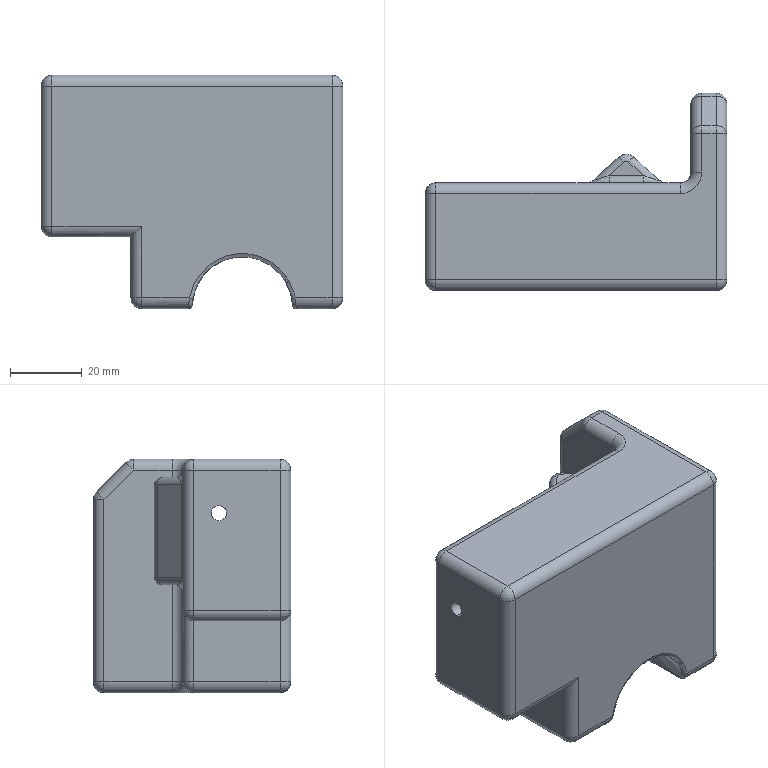Part | STEP file | PTFE block (upper) | 1 solid | 101 faces | box 84 x 55 x 65 mm | volume 139929 mm3 | cylinder 47 | plane 19 | spline 17 | sphere 14 | torus 2 | other 2 | commonest cylinder face diameters 6 x29 4 x8 4.2 x2 10.2 x2 12 x2 14 x2